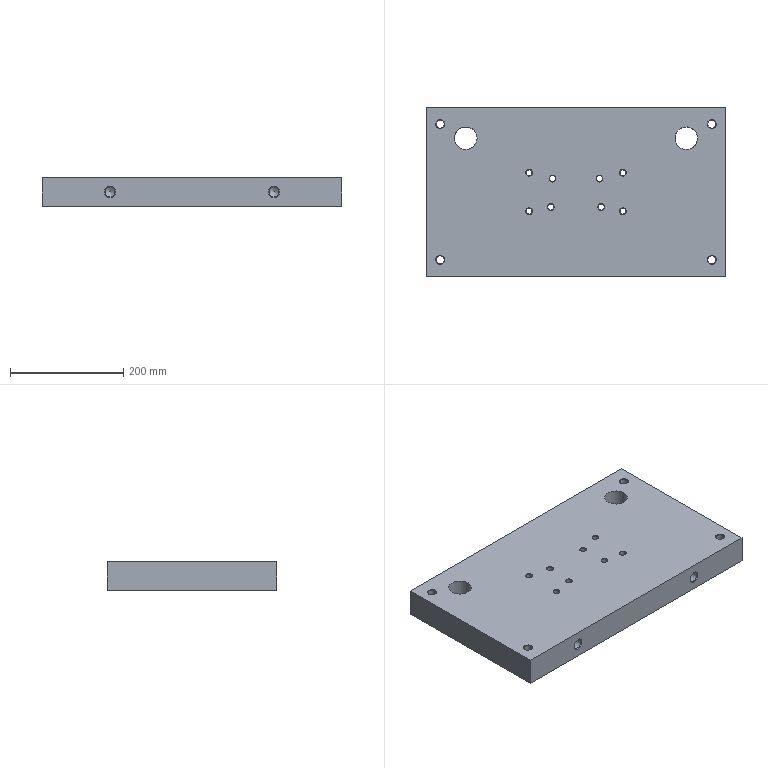Part | STEP file | gslz 2016.10.28-6_id1070_x_t | 1 solid | 134 faces | box 530 x 300 x 50 mm | volume 7668211 mm3 | cone 70 | cylinder 49 | plane 15 | commonest cylinder face diameters 6.8 x14 8.5 x8 10.5 x8 16 x6 14 x4 17.5 x4